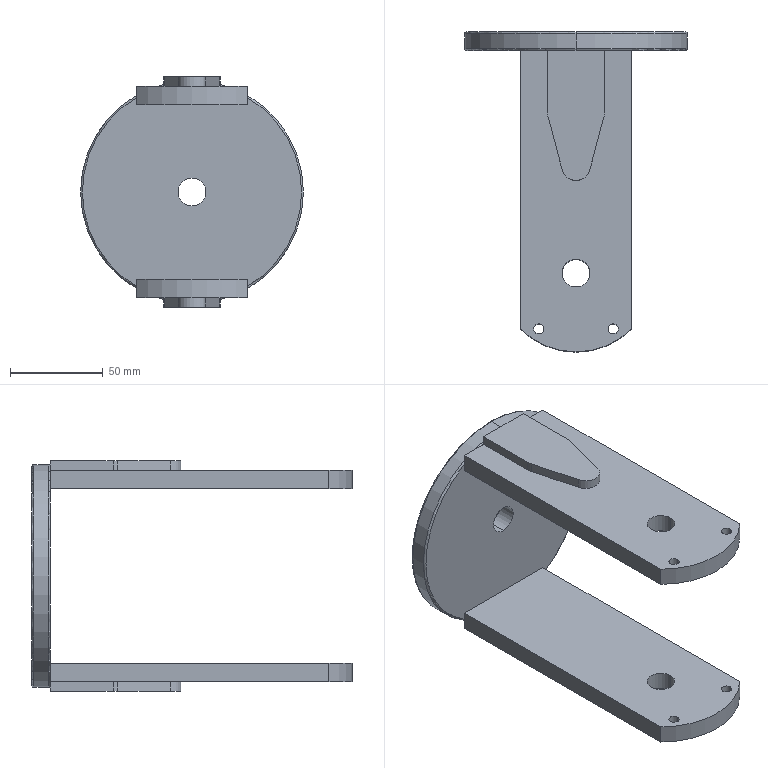Part | SolidWorks | features ICE 3, MirrorPattern 2, Extrusion 1, Fillet 1, HoleWzd 1 | 1 solid | 54 faces | box 120 x 172.426 x 124 mm | volume 314917 mm3 | plane 26 | cylinder 24 | torus 4 | commonest cylinder face diameters 5.5 x8 15 x6 20 x4 15.301 x2 84.853 x2 120 x2